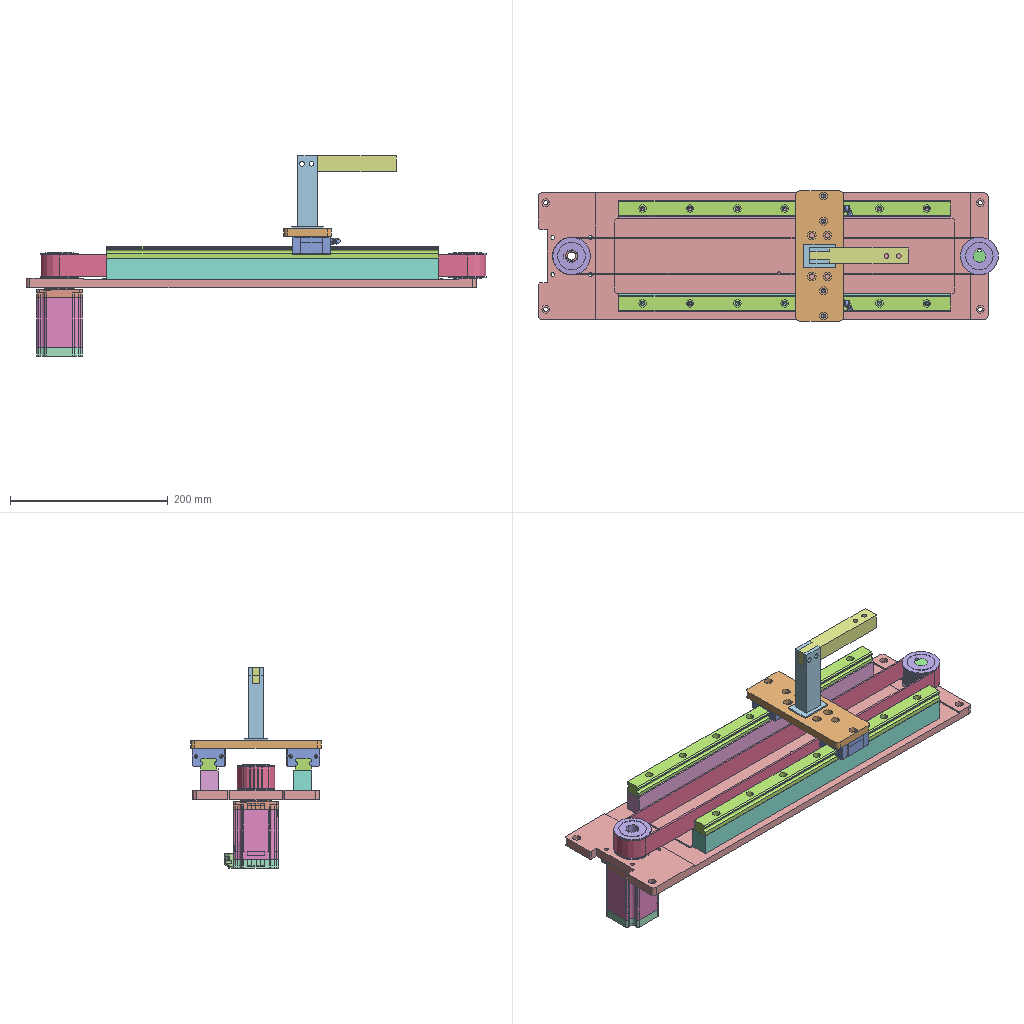Assembly | SolidWorks | 39 different items | 47 placed | box 583 x 165 x 254 mm
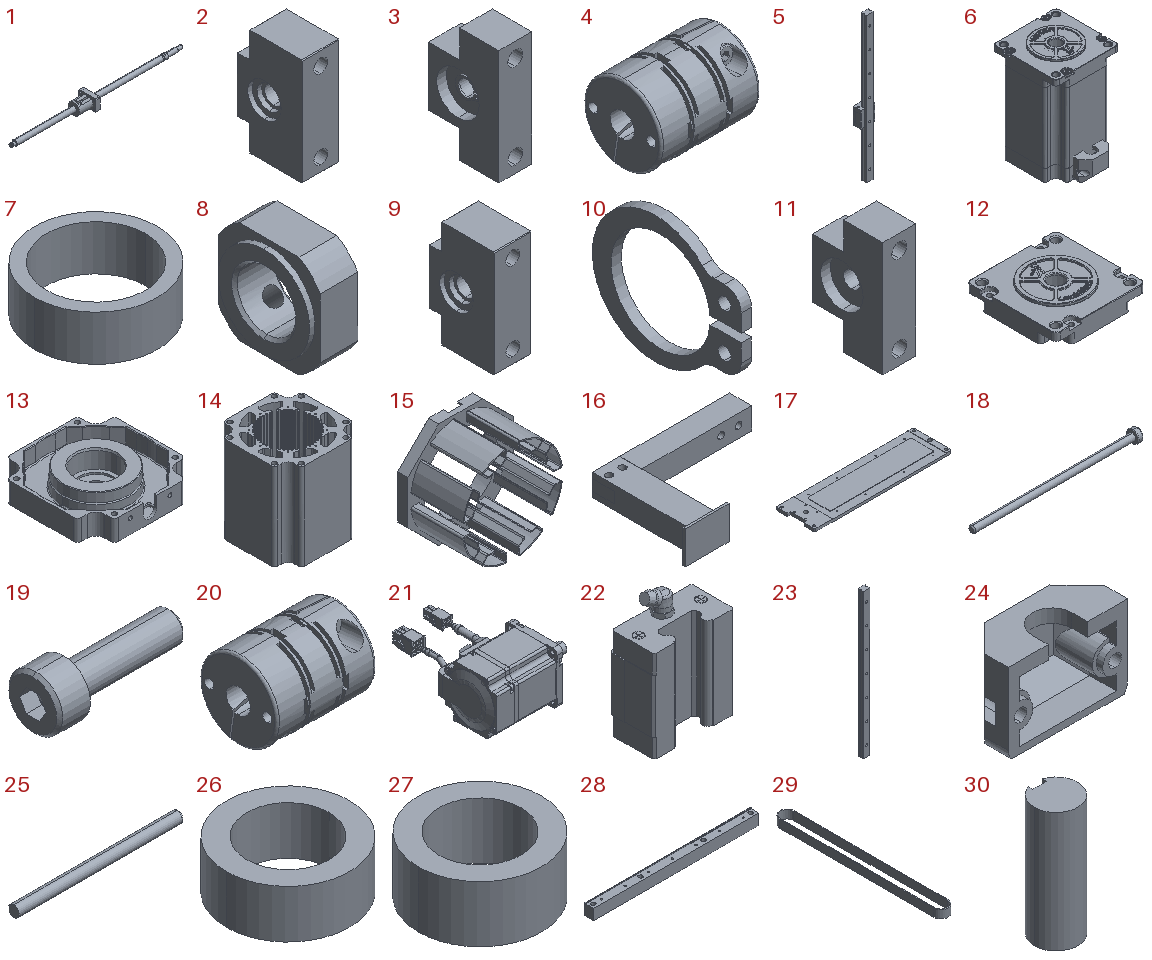Parts list (item | name | quantity | parent item | size | volume | features):
1 | (subassembly) | x1 | - | 500 x 50 x 34 mm | 126804 mm3 | -
2 | (subassembly) | x1 | - | 35.5 x 43 x 70 mm | 62101 mm3 | -
3 | (subassembly) | x1 | - | 20 x 43 x 70 mm | 37286 mm3 | -
4 | (subassembly) | x1 | - | 41 x 32 x 32 mm | 23844 mm3 | -
5 | (subassembly) | x2 | - | 42 x 28 x 420 mm | 150094 mm3 | -
6 | (subassembly) | x1 | - | - | - | -
7 | - | x1 | - | 15 x 15 x 5.5 mm | 349.895 mm3 | features BaseBody 1
8 | - | x1 | - | 8 x 19 x 19 mm | 1767 mm3 | features BaseBody 1
9 | - | x1 | - | 30 x 43 x 70 mm | 59984 mm3 | features BaseBody 1
10 | - | x1 | - | 1 x 14.4 x 12.3 mm | 59.275 mm3 | features BaseBody 1
11 | - | x1 | - | 20 x 43 x 70 mm | 37227 mm3 | features BaseBody 1
12 | - | x1 | in 6 | - | - | features RefSurface 1
13 | - | x1 | in 6 | - | - | features RefSurface 1
14 | - | x1 | in 6 | - | - | features RefSurface 1
15 | - | x2 | in 6 | - | - | features RefSurface 1
16 | - | x1 | - | 132.5 x 92 x 30 mm | 85138 mm3 | features Cut 3, ICE 2, Extrusion 1
17 | - | x1 | - | 570 x 160 x 12 mm | 1005956 mm3 | features Cut 3, ICE 3, Fillet 2, HoleWzd 2, Chamfer 1, Extrusion 1
18 | - | x4 | in 6 | - | - | features RefSurface 1
19 | - | x1 | - | 18 x 7 x 7 mm | 310.563 mm3 | features BaseBody 1
20 | - | x1 | - | 41 x 32 x 32 mm | 23223 mm3 | features BaseBody 1
21 | - | x1 | - | 109.5 x 145.682 x 60 mm | 283443 mm3 | features BaseBody 7
22 | - | x2 | in 5 | 42 x 22.5 x 60 mm | 34843 mm3 | features BaseBody 1
23 | - | x2 | in 5 | 20 x 15.5 x 420 mm | 115251 mm3 | features BaseBody 1
24 | - | x1 | in 6 | - | - | features RefSurface 1
25 | - | x1 | - | - | - | features RefSurface 1
26 | - | x1 | - | - | - | features RefSurface 1
27 | - | x1 | - | - | - | features RefSurface 1
28 | - | x1 | - | 420 x 22 x 29 mm | 243626 mm3 | features HoleWzd 2, Extrusion 1, ICE 1
29 | - | x1 | - | 47.9 x 564.4 x 27 mm | 68430 mm3 | features CompositeCurve 1, Extrusion 1, ICE 1
30 | - | x1 | - | 16 x 15.599 x 44 mm | 8436 mm3 | features Extrusion 1
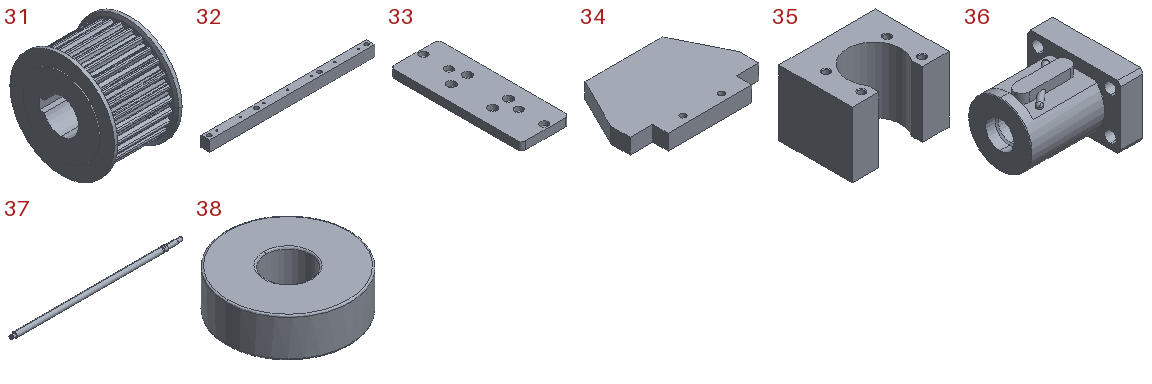31 | - | x2 | - | 32 x 47.9 x 47.9 mm | 37659 mm3 | features RevCut 8, ICE 5, Revolution 3, Fillet 2, CirPattern 1
32 | - | x1 | - | 420 x 22 x 27 mm | 241946 mm3 | features HoleWzd 2, Extrusion 1
33 | - | x1 | - | 60 x 165 x 10 mm | 93726 mm3 | features HoleWzd 2, Extrusion 1, Fillet 1
34 | - | x1 | - | 100 x 67 x 12 mm | 65076 mm3 | features Chamfer 2, Extrusion 1, HoleWzd 1, ICE 1
35 | - | x1 | - | 62 x 47 x 42 mm | 79435 mm3 | features BaseBody 1
36 | - | x1 | - | 52 x 50 x 34 mm | 43614 mm3 | features BaseBody 1
37 | - | x1 | - | 500 x 15 x 15 mm | 83191 mm3 | features BaseBody 1
38 | - | x1 | - | - | - | features RefSurface 1
39 | ZZ57HS076DF038X-S2_1 (subassembly) | x1 | - | - | - | -
Mates (type | each side: item.copy, entity, surface, feature):
In the top assembly
Coincident | 17.1 face plane Cut-Extrude1 | 28.1 face plane Boss-Extrude1
Coincident | 17.1 face plane Cut-Extrude2 | 28.1 face plane Boss-Extrude1
Coincident | 23.1 face plane _SVRL28_420_r | 28.1 face plane Boss-Extrude1
Coincident | 23.2 face plane _SVRL28_420_r | 28.1 face plane Boss-Extrude1 | 2 times
Coincident | 23.2 face plane _SVRL28_420_r | 28.1 face plane Boss-Extrude2
Coincident | 17.1 face plane Cut-Extrude1 | 32.1 face plane Boss-Extrude1
Coincident | 17.1 edge | 32.1 face plane Boss-Extrude1
Coincident | 23.1 face plane _SVRL28_420_r | 32.1 face plane Boss-Extrude1 | 2 times
DistanceDim | 23.1 face plane _SVRL28_420_r | 32.1 face plane Boss-Extrude1
Coincident | 22.1 face plane _SVR28_b | 22.2 face plane _SVR28_b
Coincident | 17.1 face plane Boss-Extrude1 | 31.1 face plane Revolve1
Concentric | 17.1 face cylinder Cut-Extrude4 | 31.1 face cylinder Cut-Extrude4
Parallel | 17.1 face plane Cut-Extrude3 | 31.1 face plane Cut-Extrude4
Coincident | 17.1 face plane Boss-Extrude1 | 12.1 face plane Surface-Input1
Concentric | assembly face | 31.1 face cylinder Cut-Extrude4
Parallel | 17.1 face plane Cut-Extrude3 | 14.1 face plane Surface-Input1
Coincident | 17.1 face plane Boss-Extrude1 | 31.2 face plane Revolve1
Concentric | 17.1 face cylinder Cut-Extrude6 | 31.2 face cylinder Cut-Extrude4
InPlace | 17.1 face plane Boss-Extrude1 | 30.1 plane
InPlace | 31.1 face plane Revolve3 | 29.1 plane
Coincident | 22.1 face plane _SVR28_b | 33.1 face plane Boss-Extrude1
In subassembly 5
DistanceDim | 22.3 face plane _SVR28_b | 23.3 face plane _SVRL28_420_r | 2 times